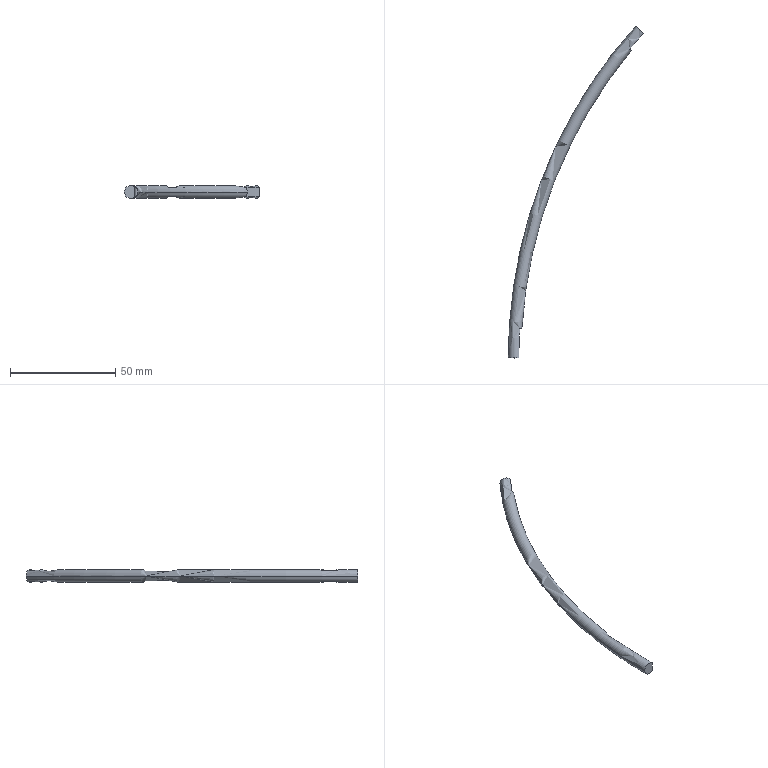Part | SolidWorks | features ICE 1, Sweep 1 | 1 solid | 8 faces | box 64.334 x 157.915 x 6 mm | volume 4754 mm3 | plane 4 | torus 2 | cylinder 2 | commonest cylinder face diameters 462 x2
STEP:
#1=CARTESIAN_POINT('',(-171.666,154.569,2.236));
#2=VERTEX_POINT('',#1);
#3=CARTESIAN_POINT('',(-175.382,157.915,0.));
#4=VERTEX_POINT('',#3);
#5=CARTESIAN_POINT('',(-173.153,155.907,0.));
#6=DIRECTION('',(-0.6691,-0.7431,0.));
#7=DIRECTION('',(0.7431,-0.6691,0.));
#8=AXIS2_PLACEMENT_3D('',#5,#6,#7);
#9=CIRCLE('',#8,3.);
#10=EDGE_CURVE('',#2,#4,#9,.T.);
#11=ORIENTED_EDGE('',*,*,#10,.T.);
#12=CARTESIAN_POINT('',(-236.,0.,0.));
#13=VERTEX_POINT('',#12);
#14=CARTESIAN_POINT('',(0.,0.,0.));
#15=DIRECTION('',(0.,0.,1.));
#16=DIRECTION('',(1.,0.,0.));
#17=AXIS2_PLACEMENT_3D('',#14,#15,#16);
#18=CIRCLE('',#17,236.);
#19=EDGE_CURVE('',#4,#13,#18,.T.);
#20=ORIENTED_EDGE('',*,*,#19,.T.);
#21=CARTESIAN_POINT('',(-231.,0.,2.236));
#22=VERTEX_POINT('',#21);
#23=CARTESIAN_POINT('',(-233.,0.,0.));
#24=DIRECTION('',(0.,-1.,0.));
#25=DIRECTION('',(1.,0.,0.));
#26=AXIS2_PLACEMENT_3D('',#23,#24,#25);
#27=CIRCLE('',#26,3.);
#28=EDGE_CURVE('',#22,#13,#27,.T.);
#29=ORIENTED_EDGE('',*,*,#28,.F.);
#30=CARTESIAN_POINT('',(-230.569,14.102,2.236));
#31=VERTEX_POINT('',#30);
#32=CARTESIAN_POINT('',(0.,0.,2.236));
#33=DIRECTION('',(0.,0.,1.));
#34=DIRECTION('',(-1.,0.,0.));
#35=AXIS2_PLACEMENT_3D('',#32,#33,#34);
#36=CIRCLE('',#35,231.);
#37=EDGE_CURVE('',#31,#22,#36,.T.);
#38=ORIENTED_EDGE('',*,*,#37,.F.);
#39=CARTESIAN_POINT('',(-229.571,14.041,0.));
#40=VERTEX_POINT('',#39);
#41=CARTESIAN_POINT('',(-232.565,14.224,0.));
#42=DIRECTION('',(-0.06105,-0.9981,0.));
#43=DIRECTION('',(-0.9981,0.06105,0.));
#44=AXIS2_PLACEMENT_3D('',#41,#42,#43);
#45=CIRCLE('',#44,3.);
#46=EDGE_CURVE('',#40,#31,#45,.T.);
#47=ORIENTED_EDGE('',*,*,#46,.F.);
#48=CARTESIAN_POINT('',(-177.474,146.298,0.));
#49=VERTEX_POINT('',#48);
#50=CARTESIAN_POINT('',(0.,0.,0.));
#51=DIRECTION('',(0.,0.,1.));
#52=DIRECTION('',(1.,0.,0.));
#53=AXIS2_PLACEMENT_3D('',#50,#51,#52);
#54=CIRCLE('',#53,230.);
#55=EDGE_CURVE('',#49,#40,#54,.T.);
#56=ORIENTED_EDGE('',*,*,#55,.F.);
#57=CARTESIAN_POINT('',(-178.245,146.934,2.236));
#58=VERTEX_POINT('',#57);
#59=CARTESIAN_POINT('',(-179.789,148.206,0.));
#60=DIRECTION('',(-0.6361,-0.7716,0.));
#61=DIRECTION('',(-0.7716,0.6361,0.));
#62=AXIS2_PLACEMENT_3D('',#59,#60,#61);
#63=CIRCLE('',#62,3.);
#64=EDGE_CURVE('',#49,#58,#63,.T.);
#65=ORIENTED_EDGE('',*,*,#64,.T.);
#66=CARTESIAN_POINT('',(0.,0.,2.236));
#67=DIRECTION('',(0.,0.,1.));
#68=DIRECTION('',(-1.,0.,0.));
#69=AXIS2_PLACEMENT_3D('',#66,#67,#68);
#70=CIRCLE('',#69,231.);
#71=EDGE_CURVE('',#2,#58,#70,.T.);
#72=ORIENTED_EDGE('',*,*,#71,.F.);
#73=EDGE_LOOP('',(#11,#20,#29,#38,#47,#56,#65,#72));
#74=FACE_OUTER_BOUND('',#73,.T.);
#75=CARTESIAN_POINT('',(0.,0.,0.));
#76=DIRECTION('',(0.,0.,1.));
#77=DIRECTION('',(1.,0.,0.));
#78=AXIS2_PLACEMENT_3D('',#75,#76,#77);
#79=TOROIDAL_SURFACE('',#78,233.,3.);
#80=ADVANCED_FACE('',(#74),#79,.T.);
#81=ORIENTED_EDGE('',*,*,#19,.F.);
#82=CARTESIAN_POINT('',(-171.666,154.569,-2.236));
#83=VERTEX_POINT('',#82);
#84=CARTESIAN_POINT('',(-173.153,155.907,0.));
#85=DIRECTION('',(-0.6691,-0.7431,0.));
#86=DIRECTION('',(0.7431,-0.6691,0.));
#87=AXIS2_PLACEMENT_3D('',#84,#85,#86);
#88=CIRCLE('',#87,3.);
#89=EDGE_CURVE('',#4,#83,#88,.T.);
#90=ORIENTED_EDGE('',*,*,#89,.T.);
#91=CARTESIAN_POINT('',(-178.245,146.934,-2.236));
#92=VERTEX_POINT('',#91);
#93=CARTESIAN_POINT('',(0.,0.,-2.236));
#94=DIRECTION('',(0.,0.,-1.));
#95=DIRECTION('',(1.,0.,0.));
#96=AXIS2_PLACEMENT_3D('',#93,#94,#95);
#97=CIRCLE('',#96,231.);
#98=EDGE_CURVE('',#92,#83,#97,.T.);
#99=ORIENTED_EDGE('',*,*,#98,.F.);
#100=CARTESIAN_POINT('',(-179.789,148.206,0.));
#101=DIRECTION('',(-0.6361,-0.7716,0.));
#102=DIRECTION('',(-0.7716,0.6361,0.));
#103=AXIS2_PLACEMENT_3D('',#100,#101,#102);
#104=CIRCLE('',#103,3.);
#105=EDGE_CURVE('',#92,#49,#104,.T.);
#106=ORIENTED_EDGE('',*,*,#105,.T.);
#107=ORIENTED_EDGE('',*,*,#55,.T.);
#108=CARTESIAN_POINT('',(-230.569,14.102,-2.236));
#109=VERTEX_POINT('',#108);
#110=CARTESIAN_POINT('',(-232.565,14.224,0.));
#111=DIRECTION('',(-0.06105,-0.9981,0.));
#112=DIRECTION('',(-0.9981,0.06105,0.));
#113=AXIS2_PLACEMENT_3D('',#110,#111,#112);
#114=CIRCLE('',#113,3.);
#115=EDGE_CURVE('',#109,#40,#114,.T.);
#116=ORIENTED_EDGE('',*,*,#115,.F.);
#117=CARTESIAN_POINT('',(-231.,0.,-2.236));
#118=VERTEX_POINT('',#117);
#119=CARTESIAN_POINT('',(0.,0.,-2.236));
#120=DIRECTION('',(0.,0.,-1.));
#121=DIRECTION('',(1.,0.,0.));
#122=AXIS2_PLACEMENT_3D('',#119,#120,#121);
#123=CIRCLE('',#122,231.);
#124=EDGE_CURVE('',#118,#109,#123,.T.);
#125=ORIENTED_EDGE('',*,*,#124,.F.);
#126=CARTESIAN_POINT('',(-233.,0.,0.));
#127=DIRECTION('',(0.,-1.,0.));
#128=DIRECTION('',(1.,0.,0.));
#129=AXIS2_PLACEMENT_3D('',#126,#127,#128);
#130=CIRCLE('',#129,3.);
#131=EDGE_CURVE('',#13,#118,#130,.T.);
#132=ORIENTED_EDGE('',*,*,#131,.F.);
#133=EDGE_LOOP('',(#81,#90,#99,#106,#107,#116,#125,#132));
#134=FACE_OUTER_BOUND('',#133,.T.);
#135=CARTESIAN_POINT('',(0.,0.,0.));
#136=DIRECTION('',(0.,0.,1.));
#137=DIRECTION('',(1.,0.,0.));
#138=AXIS2_PLACEMENT_3D('',#135,#136,#137);
#139=TOROIDAL_SURFACE('',#138,233.,3.);
#140=ADVANCED_FACE('',(#134),#139,.T.);
#141=CARTESIAN_POINT('',(-231.,0.,-25.));
#142=DIRECTION('',(0.,0.,1.));
#143=VECTOR('',#142,1000.);
#144=LINE('',#141,#143);
#145=EDGE_CURVE('',#118,#22,#144,.T.);
#146=ORIENTED_EDGE('',*,*,#145,.T.);
#147=ORIENTED_EDGE('',*,*,#28,.T.);
#148=ORIENTED_EDGE('',*,*,#131,.T.);
#149=EDGE_LOOP('',(#146,#147,#148));
#150=FACE_OUTER_BOUND('',#149,.T.);
#151=CARTESIAN_POINT('',(-233.,0.,0.));
#152=DIRECTION('',(0.,-1.,0.));
#153=DIRECTION('',(1.,0.,0.));
#154=AXIS2_PLACEMENT_3D('',#151,#152,#153);
#155=PLANE('',#154);
#156=ADVANCED_FACE('',(#150),#155,.T.);
#157=ORIENTED_EDGE('',*,*,#10,.F.);
#158=CARTESIAN_POINT('',(-171.666,154.569,-25.));
#159=DIRECTION('',(0.,0.,1.));
#160=VECTOR('',#159,1000.);
#161=LINE('',#158,#160);
#162=EDGE_CURVE('',#83,#2,#161,.T.);
#163=ORIENTED_EDGE('',*,*,#162,.F.);
#164=ORIENTED_EDGE('',*,*,#89,.F.);
#165=EDGE_LOOP('',(#157,#163,#164));
#166=FACE_OUTER_BOUND('',#165,.T.);
#167=CARTESIAN_POINT('',(-173.153,155.907,0.));
#168=DIRECTION('',(-0.6691,-0.7431,0.));
#169=DIRECTION('',(0.7431,-0.6691,0.));
#170=AXIS2_PLACEMENT_3D('',#167,#168,#169);
#171=PLANE('',#170);
#172=ADVANCED_FACE('',(#166),#171,.F.);
#173=ORIENTED_EDGE('',*,*,#115,.T.);
#174=ORIENTED_EDGE('',*,*,#46,.T.);
#175=CARTESIAN_POINT('',(-230.569,14.102,-25.));
#176=DIRECTION('',(0.,0.,1.));
#177=VECTOR('',#176,1000.);
#178=LINE('',#175,#177);
#179=EDGE_CURVE('',#109,#31,#178,.T.);
#180=ORIENTED_EDGE('',*,*,#179,.F.);
#181=EDGE_LOOP('',(#173,#174,#180));
#182=FACE_OUTER_BOUND('',#181,.T.);
#183=CARTESIAN_POINT('',(0.,0.,-25.));
#184=DIRECTION('',(0.06105,0.9981,0.));
#185=DIRECTION('',(-0.9981,0.06105,0.));
#186=AXIS2_PLACEMENT_3D('',#183,#184,#185);
#187=PLANE('',#186);
#188=ADVANCED_FACE('',(#182),#187,.F.);
#189=ORIENTED_EDGE('',*,*,#37,.T.);
#190=ORIENTED_EDGE('',*,*,#145,.F.);
#191=ORIENTED_EDGE('',*,*,#124,.T.);
#192=ORIENTED_EDGE('',*,*,#179,.T.);
#193=EDGE_LOOP('',(#189,#190,#191,#192));
#194=FACE_OUTER_BOUND('',#193,.T.);
#195=CARTESIAN_POINT('',(0.,0.,-25.));
#196=DIRECTION('',(0.,0.,1.));
#197=DIRECTION('',(1.,0.,0.));
#198=AXIS2_PLACEMENT_3D('',#195,#196,#197);
#199=CYLINDRICAL_SURFACE('',#198,231.);
#200=ADVANCED_FACE('',(#194),#199,.F.);
#201=CARTESIAN_POINT('',(-178.245,146.934,-25.));
#202=DIRECTION('',(0.,0.,1.));
#203=VECTOR('',#202,1000.);
#204=LINE('',#201,#203);
#205=EDGE_CURVE('',#92,#58,#204,.T.);
#206=ORIENTED_EDGE('',*,*,#205,.T.);
#207=ORIENTED_EDGE('',*,*,#64,.F.);
#208=ORIENTED_EDGE('',*,*,#105,.F.);
#209=EDGE_LOOP('',(#206,#207,#208));
#210=FACE_OUTER_BOUND('',#209,.T.);
#211=CARTESIAN_POINT('',(0.,0.,-25.));
#212=DIRECTION('',(0.6361,0.7716,0.));
#213=DIRECTION('',(-0.7716,0.6361,0.));
#214=AXIS2_PLACEMENT_3D('',#211,#212,#213);
#215=PLANE('',#214);
#216=ADVANCED_FACE('',(#210),#215,.T.);
#217=ORIENTED_EDGE('',*,*,#71,.T.);
#218=ORIENTED_EDGE('',*,*,#205,.F.);
#219=ORIENTED_EDGE('',*,*,#98,.T.);
#220=ORIENTED_EDGE('',*,*,#162,.T.);
#221=EDGE_LOOP('',(#217,#218,#219,#220));
#222=FACE_OUTER_BOUND('',#221,.T.);
#223=CARTESIAN_POINT('',(0.,0.,-25.));
#224=DIRECTION('',(0.,0.,1.));
#225=DIRECTION('',(1.,0.,0.));
#226=AXIS2_PLACEMENT_3D('',#223,#224,#225);
#227=CYLINDRICAL_SURFACE('',#226,231.);
#228=ADVANCED_FACE('',(#222),#227,.F.);
#229=CLOSED_SHELL('',(#80,#140,#156,#172,#188,#200,#216,#228));
#230=MANIFOLD_SOLID_BREP('',#229);
#231=CARTESIAN_POINT('',(0.,0.,0.));
#232=DIRECTION('',(0.,0.,1.));
#233=DIRECTION('',(1.,0.,0.));
#234=AXIS2_PLACEMENT_3D('',#231,#232,#233);
#235=(LENGTH_UNIT()NAMED_UNIT(*)SI_UNIT(.MILLI.,.METRE.));
#236=UNCERTAINTY_MEASURE_WITH_UNIT(LENGTH_MEASURE(0.00001),#235,'','');
#237=(NAMED_UNIT(*)PLANE_ANGLE_UNIT()SI_UNIT($,.RADIAN.));
#238=(NAMED_UNIT(*)SI_UNIT($,.STERADIAN.)SOLID_ANGLE_UNIT());
#239=(GEOMETRIC_REPRESENTATION_CONTEXT(3)GLOBAL_UNCERTAINTY_ASSIGNED_CONTEXT((#236))GLOBAL_UNIT_ASSIGNED_CONTEXT((#235,#237,#238))REPRESENTATION_CONTEXT('',''));
#240=ADVANCED_BREP_SHAPE_REPRESENTATION('',(#230,#234),#239);